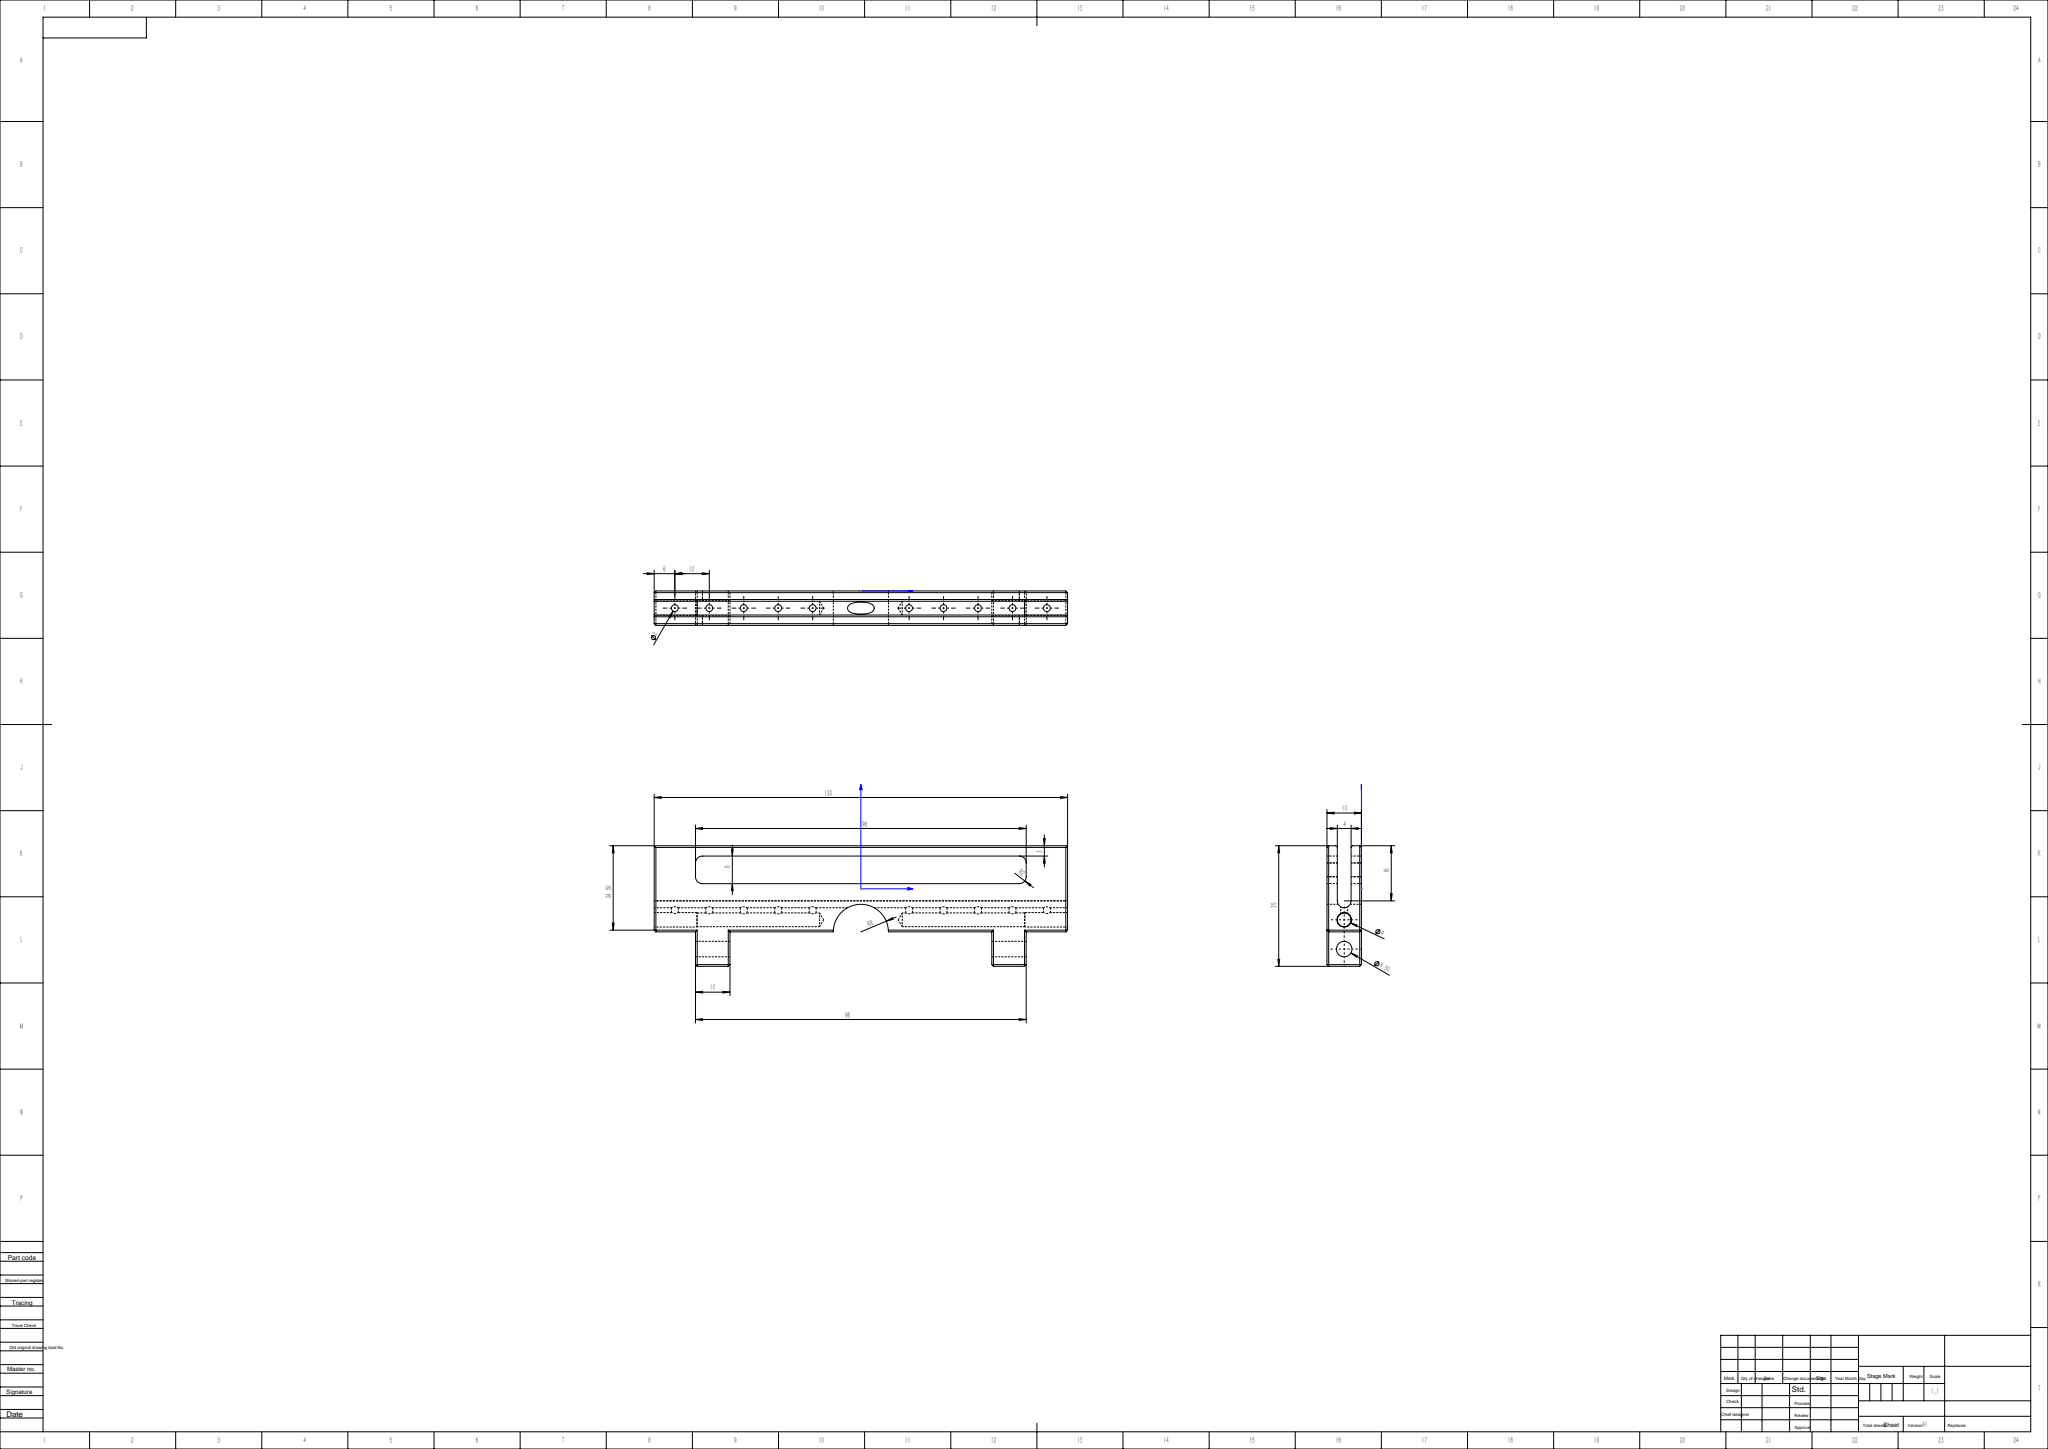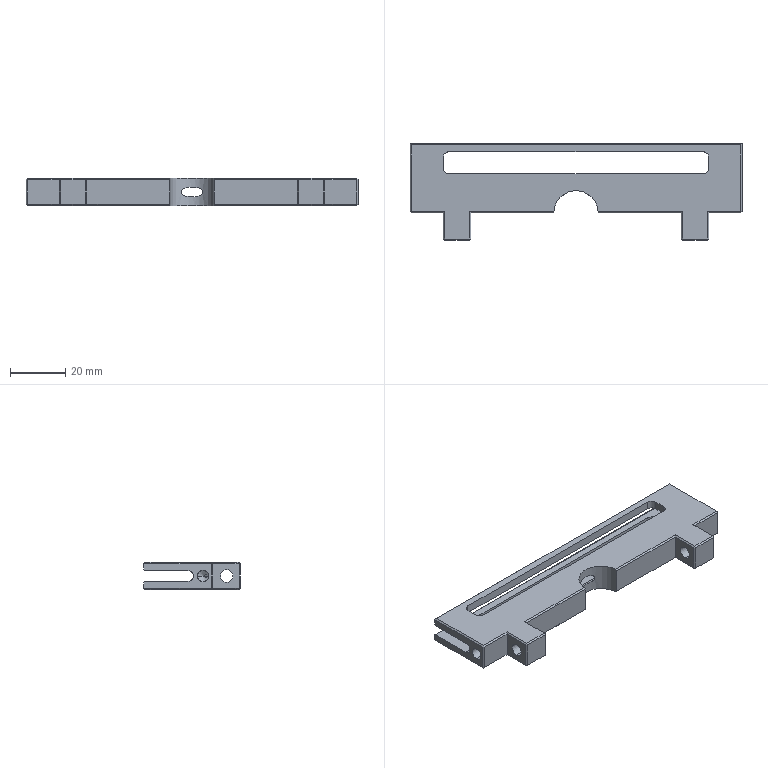Part | SolidWorks | features BaseBody 1 | 1 solid | 122 faces | box 120 x 35 x 10 mm | volume 16270 mm3 | plane 70 | cylinder 44 | cone 8 | commonest cylinder face diameters 2 x20 4 x13 4.2 x4 4.5 x4 1 x2 16 x1